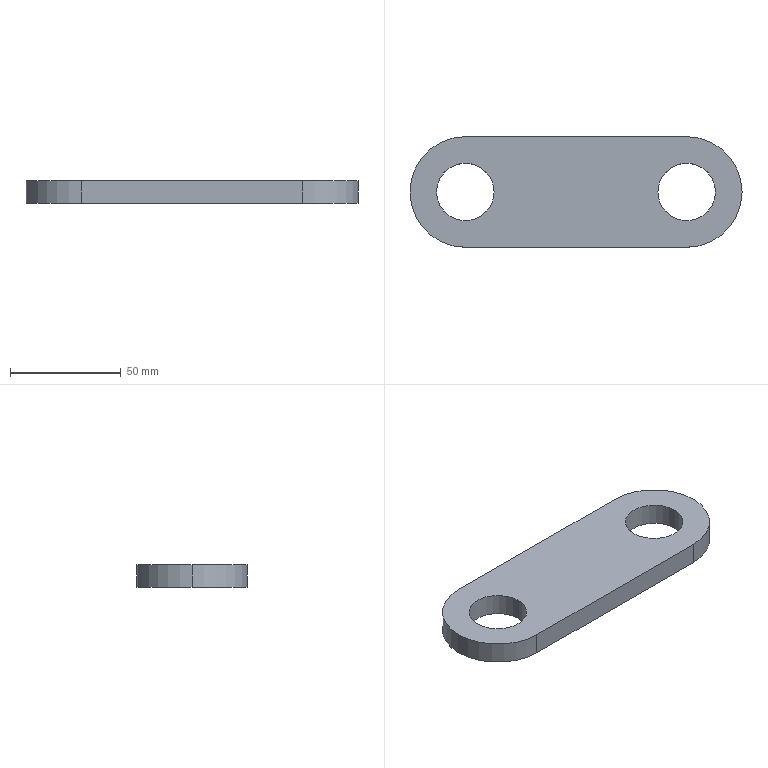Part | STEP file | MYT-A01-P16 | 1 solid | 11 faces | box 150 x 50 x 10 mm | volume 59016 mm3 | cylinder 7 | plane 4 | commonest cylinder face diameters 26 x4 50 x3
STEP:
#1=CARTESIAN_POINT('',(-13.,0.,0.));
#2=VERTEX_POINT('',#1);
#3=CARTESIAN_POINT('',(13.,0.,0.));
#4=VERTEX_POINT('',#3);
#5=CARTESIAN_POINT('',(0.,0.,0.));
#6=DIRECTION('',(0.,0.,1.));
#7=DIRECTION('',(1.,0.,0.));
#8=AXIS2_PLACEMENT_3D('',#5,#6,#7);
#9=CIRCLE('',#8,13.);
#10=EDGE_CURVE('',#2,#4,#9,.T.);
#11=ORIENTED_EDGE('',*,*,#10,.F.);
#12=CARTESIAN_POINT('',(-13.,0.,10.));
#13=VERTEX_POINT('',#12);
#14=CARTESIAN_POINT('',(-13.,0.,0.));
#15=DIRECTION('',(0.,0.,1.));
#16=VECTOR('',#15,1000.);
#17=LINE('',#14,#16);
#18=EDGE_CURVE('',#2,#13,#17,.T.);
#19=ORIENTED_EDGE('',*,*,#18,.T.);
#20=CARTESIAN_POINT('',(13.,0.,10.));
#21=VERTEX_POINT('',#20);
#22=CARTESIAN_POINT('',(0.,0.,10.));
#23=DIRECTION('',(0.,0.,1.));
#24=DIRECTION('',(1.,0.,0.));
#25=AXIS2_PLACEMENT_3D('',#22,#23,#24);
#26=CIRCLE('',#25,13.);
#27=EDGE_CURVE('',#13,#21,#26,.T.);
#28=ORIENTED_EDGE('',*,*,#27,.T.);
#29=CARTESIAN_POINT('',(13.,0.,0.));
#30=DIRECTION('',(0.,0.,1.));
#31=VECTOR('',#30,1000.);
#32=LINE('',#29,#31);
#33=EDGE_CURVE('',#4,#21,#32,.T.);
#34=ORIENTED_EDGE('',*,*,#33,.F.);
#35=EDGE_LOOP('',(#11,#19,#28,#34));
#36=FACE_OUTER_BOUND('',#35,.T.);
#37=CARTESIAN_POINT('',(0.,0.,0.));
#38=DIRECTION('',(0.,0.,1.));
#39=DIRECTION('',(1.,0.,0.));
#40=AXIS2_PLACEMENT_3D('',#37,#38,#39);
#41=CYLINDRICAL_SURFACE('',#40,13.);
#42=ADVANCED_FACE('',(#36),#41,.F.);
#43=CARTESIAN_POINT('',(87.,0.,0.));
#44=VERTEX_POINT('',#43);
#45=CARTESIAN_POINT('',(113.,0.,0.));
#46=VERTEX_POINT('',#45);
#47=CARTESIAN_POINT('',(100.,0.,0.));
#48=DIRECTION('',(0.,0.,1.));
#49=DIRECTION('',(1.,0.,0.));
#50=AXIS2_PLACEMENT_3D('',#47,#48,#49);
#51=CIRCLE('',#50,13.);
#52=EDGE_CURVE('',#44,#46,#51,.T.);
#53=ORIENTED_EDGE('',*,*,#52,.F.);
#54=CARTESIAN_POINT('',(87.,0.,10.));
#55=VERTEX_POINT('',#54);
#56=CARTESIAN_POINT('',(87.,0.,0.));
#57=DIRECTION('',(0.,0.,1.));
#58=VECTOR('',#57,1000.);
#59=LINE('',#56,#58);
#60=EDGE_CURVE('',#44,#55,#59,.T.);
#61=ORIENTED_EDGE('',*,*,#60,.T.);
#62=CARTESIAN_POINT('',(113.,0.,10.));
#63=VERTEX_POINT('',#62);
#64=CARTESIAN_POINT('',(100.,0.,10.));
#65=DIRECTION('',(0.,0.,1.));
#66=DIRECTION('',(1.,0.,0.));
#67=AXIS2_PLACEMENT_3D('',#64,#65,#66);
#68=CIRCLE('',#67,13.);
#69=EDGE_CURVE('',#55,#63,#68,.T.);
#70=ORIENTED_EDGE('',*,*,#69,.T.);
#71=CARTESIAN_POINT('',(113.,0.,0.));
#72=DIRECTION('',(0.,0.,1.));
#73=VECTOR('',#72,1000.);
#74=LINE('',#71,#73);
#75=EDGE_CURVE('',#46,#63,#74,.T.);
#76=ORIENTED_EDGE('',*,*,#75,.F.);
#77=EDGE_LOOP('',(#53,#61,#70,#76));
#78=FACE_OUTER_BOUND('',#77,.T.);
#79=CARTESIAN_POINT('',(100.,0.,0.));
#80=DIRECTION('',(0.,0.,1.));
#81=DIRECTION('',(1.,0.,0.));
#82=AXIS2_PLACEMENT_3D('',#79,#80,#81);
#83=CYLINDRICAL_SURFACE('',#82,13.);
#84=ADVANCED_FACE('',(#78),#83,.F.);
#85=CARTESIAN_POINT('',(-25.,0.,10.));
#86=VERTEX_POINT('',#85);
#87=CARTESIAN_POINT('',(0.,-25.,10.));
#88=VERTEX_POINT('',#87);
#89=CARTESIAN_POINT('',(0.,0.,10.));
#90=DIRECTION('',(0.,0.,1.));
#91=DIRECTION('',(1.,0.,0.));
#92=AXIS2_PLACEMENT_3D('',#89,#90,#91);
#93=CIRCLE('',#92,25.);
#94=EDGE_CURVE('',#86,#88,#93,.T.);
#95=ORIENTED_EDGE('',*,*,#94,.F.);
#96=CARTESIAN_POINT('',(-25.,0.,0.));
#97=VERTEX_POINT('',#96);
#98=CARTESIAN_POINT('',(-25.,0.,10.));
#99=DIRECTION('',(0.,0.,-1.));
#100=VECTOR('',#99,1000.);
#101=LINE('',#98,#100);
#102=EDGE_CURVE('',#86,#97,#101,.T.);
#103=ORIENTED_EDGE('',*,*,#102,.T.);
#104=CARTESIAN_POINT('',(0.,-25.,0.));
#105=VERTEX_POINT('',#104);
#106=CARTESIAN_POINT('',(0.,0.,0.));
#107=DIRECTION('',(0.,0.,1.));
#108=DIRECTION('',(1.,0.,0.));
#109=AXIS2_PLACEMENT_3D('',#106,#107,#108);
#110=CIRCLE('',#109,25.);
#111=EDGE_CURVE('',#97,#105,#110,.T.);
#112=ORIENTED_EDGE('',*,*,#111,.T.);
#113=CARTESIAN_POINT('',(0.,-25.,10.));
#114=DIRECTION('',(0.,0.,-1.));
#115=VECTOR('',#114,1000.);
#116=LINE('',#113,#115);
#117=EDGE_CURVE('',#88,#105,#116,.T.);
#118=ORIENTED_EDGE('',*,*,#117,.F.);
#119=EDGE_LOOP('',(#95,#103,#112,#118));
#120=FACE_OUTER_BOUND('',#119,.T.);
#121=CARTESIAN_POINT('',(0.,0.,10.));
#122=DIRECTION('',(0.,0.,-1.));
#123=DIRECTION('',(-1.,0.,0.));
#124=AXIS2_PLACEMENT_3D('',#121,#122,#123);
#125=CYLINDRICAL_SURFACE('',#124,25.);
#126=ADVANCED_FACE('',(#120),#125,.T.);
#127=ORIENTED_EDGE('',*,*,#102,.F.);
#128=CARTESIAN_POINT('',(0.,25.,10.));
#129=VERTEX_POINT('',#128);
#130=CARTESIAN_POINT('',(0.,0.,10.));
#131=DIRECTION('',(0.,0.,1.));
#132=DIRECTION('',(1.,0.,0.));
#133=AXIS2_PLACEMENT_3D('',#130,#131,#132);
#134=CIRCLE('',#133,25.);
#135=EDGE_CURVE('',#129,#86,#134,.T.);
#136=ORIENTED_EDGE('',*,*,#135,.F.);
#137=CARTESIAN_POINT('',(0.,25.,0.));
#138=VERTEX_POINT('',#137);
#139=CARTESIAN_POINT('',(0.,25.,10.));
#140=DIRECTION('',(0.,0.,-1.));
#141=VECTOR('',#140,1000.);
#142=LINE('',#139,#141);
#143=EDGE_CURVE('',#129,#138,#142,.T.);
#144=ORIENTED_EDGE('',*,*,#143,.T.);
#145=CARTESIAN_POINT('',(0.,0.,0.));
#146=DIRECTION('',(0.,0.,1.));
#147=DIRECTION('',(1.,0.,0.));
#148=AXIS2_PLACEMENT_3D('',#145,#146,#147);
#149=CIRCLE('',#148,25.);
#150=EDGE_CURVE('',#138,#97,#149,.T.);
#151=ORIENTED_EDGE('',*,*,#150,.T.);
#152=EDGE_LOOP('',(#127,#136,#144,#151));
#153=FACE_OUTER_BOUND('',#152,.T.);
#154=CARTESIAN_POINT('',(0.,0.,10.));
#155=DIRECTION('',(0.,0.,-1.));
#156=DIRECTION('',(-1.,0.,0.));
#157=AXIS2_PLACEMENT_3D('',#154,#155,#156);
#158=CYLINDRICAL_SURFACE('',#157,25.);
#159=ADVANCED_FACE('',(#153),#158,.T.);
#160=CARTESIAN_POINT('',(100.,-25.,0.));
#161=VERTEX_POINT('',#160);
#162=CARTESIAN_POINT('',(0.,-25.,0.));
#163=DIRECTION('',(1.,0.,0.));
#164=VECTOR('',#163,1000.);
#165=LINE('',#162,#164);
#166=EDGE_CURVE('',#105,#161,#165,.T.);
#167=ORIENTED_EDGE('',*,*,#166,.T.);
#168=CARTESIAN_POINT('',(100.,-25.,10.));
#169=VERTEX_POINT('',#168);
#170=CARTESIAN_POINT('',(100.,-25.,10.));
#171=DIRECTION('',(0.,0.,-1.));
#172=VECTOR('',#171,1000.);
#173=LINE('',#170,#172);
#174=EDGE_CURVE('',#169,#161,#173,.T.);
#175=ORIENTED_EDGE('',*,*,#174,.F.);
#176=CARTESIAN_POINT('',(0.,-25.,10.));
#177=DIRECTION('',(1.,0.,0.));
#178=VECTOR('',#177,1000.);
#179=LINE('',#176,#178);
#180=EDGE_CURVE('',#88,#169,#179,.T.);
#181=ORIENTED_EDGE('',*,*,#180,.F.);
#182=ORIENTED_EDGE('',*,*,#117,.T.);
#183=EDGE_LOOP('',(#167,#175,#181,#182));
#184=FACE_OUTER_BOUND('',#183,.T.);
#185=CARTESIAN_POINT('',(0.,-25.,10.));
#186=DIRECTION('',(0.,1.,0.));
#187=DIRECTION('',(0.,0.,1.));
#188=AXIS2_PLACEMENT_3D('',#185,#186,#187);
#189=PLANE('',#188);
#190=ADVANCED_FACE('',(#184),#189,.F.);
#191=CARTESIAN_POINT('',(100.,25.,0.));
#192=VERTEX_POINT('',#191);
#193=CARTESIAN_POINT('',(100.,0.,0.));
#194=DIRECTION('',(0.,0.,1.));
#195=DIRECTION('',(1.,0.,0.));
#196=AXIS2_PLACEMENT_3D('',#193,#194,#195);
#197=CIRCLE('',#196,25.);
#198=EDGE_CURVE('',#161,#192,#197,.T.);
#199=ORIENTED_EDGE('',*,*,#198,.T.);
#200=CARTESIAN_POINT('',(100.,25.,10.));
#201=VERTEX_POINT('',#200);
#202=CARTESIAN_POINT('',(100.,25.,10.));
#203=DIRECTION('',(0.,0.,-1.));
#204=VECTOR('',#203,1000.);
#205=LINE('',#202,#204);
#206=EDGE_CURVE('',#201,#192,#205,.T.);
#207=ORIENTED_EDGE('',*,*,#206,.F.);
#208=CARTESIAN_POINT('',(100.,0.,10.));
#209=DIRECTION('',(0.,0.,1.));
#210=DIRECTION('',(1.,0.,0.));
#211=AXIS2_PLACEMENT_3D('',#208,#209,#210);
#212=CIRCLE('',#211,25.);
#213=EDGE_CURVE('',#169,#201,#212,.T.);
#214=ORIENTED_EDGE('',*,*,#213,.F.);
#215=ORIENTED_EDGE('',*,*,#174,.T.);
#216=EDGE_LOOP('',(#199,#207,#214,#215));
#217=FACE_OUTER_BOUND('',#216,.T.);
#218=CARTESIAN_POINT('',(100.,0.,10.));
#219=DIRECTION('',(0.,0.,-1.));
#220=DIRECTION('',(-1.,0.,0.));
#221=AXIS2_PLACEMENT_3D('',#218,#219,#220);
#222=CYLINDRICAL_SURFACE('',#221,25.);
#223=ADVANCED_FACE('',(#217),#222,.T.);
#224=CARTESIAN_POINT('',(0.,25.,0.));
#225=DIRECTION('',(-1.,0.,0.));
#226=VECTOR('',#225,1000.);
#227=LINE('',#224,#226);
#228=EDGE_CURVE('',#192,#138,#227,.T.);
#229=ORIENTED_EDGE('',*,*,#228,.T.);
#230=ORIENTED_EDGE('',*,*,#143,.F.);
#231=CARTESIAN_POINT('',(0.,25.,10.));
#232=DIRECTION('',(-1.,0.,0.));
#233=VECTOR('',#232,1000.);
#234=LINE('',#231,#233);
#235=EDGE_CURVE('',#201,#129,#234,.T.);
#236=ORIENTED_EDGE('',*,*,#235,.F.);
#237=ORIENTED_EDGE('',*,*,#206,.T.);
#238=EDGE_LOOP('',(#229,#230,#236,#237));
#239=FACE_OUTER_BOUND('',#238,.T.);
#240=CARTESIAN_POINT('',(0.,25.,10.));
#241=DIRECTION('',(0.,-1.,0.));
#242=DIRECTION('',(0.,0.,-1.));
#243=AXIS2_PLACEMENT_3D('',#240,#241,#242);
#244=PLANE('',#243);
#245=ADVANCED_FACE('',(#239),#244,.F.);
#246=CARTESIAN_POINT('',(0.,0.,10.));
#247=DIRECTION('',(0.,0.,1.));
#248=DIRECTION('',(1.,0.,0.));
#249=AXIS2_PLACEMENT_3D('',#246,#247,#248);
#250=CIRCLE('',#249,13.);
#251=EDGE_CURVE('',#21,#13,#250,.T.);
#252=ORIENTED_EDGE('',*,*,#251,.F.);
#253=ORIENTED_EDGE('',*,*,#27,.F.);
#254=EDGE_LOOP('',(#252,#253));
#255=FACE_BOUND('',#254,.T.);
#256=CARTESIAN_POINT('',(100.,0.,10.));
#257=DIRECTION('',(0.,0.,1.));
#258=DIRECTION('',(1.,0.,0.));
#259=AXIS2_PLACEMENT_3D('',#256,#257,#258);
#260=CIRCLE('',#259,13.);
#261=EDGE_CURVE('',#63,#55,#260,.T.);
#262=ORIENTED_EDGE('',*,*,#261,.F.);
#263=ORIENTED_EDGE('',*,*,#69,.F.);
#264=EDGE_LOOP('',(#262,#263));
#265=FACE_BOUND('',#264,.T.);
#266=ORIENTED_EDGE('',*,*,#135,.T.);
#267=ORIENTED_EDGE('',*,*,#94,.T.);
#268=ORIENTED_EDGE('',*,*,#180,.T.);
#269=ORIENTED_EDGE('',*,*,#213,.T.);
#270=ORIENTED_EDGE('',*,*,#235,.T.);
#271=EDGE_LOOP('',(#266,#267,#268,#269,#270));
#272=FACE_OUTER_BOUND('',#271,.T.);
#273=CARTESIAN_POINT('',(0.,0.,10.));
#274=DIRECTION('',(0.,0.,1.));
#275=DIRECTION('',(1.,0.,0.));
#276=AXIS2_PLACEMENT_3D('',#273,#274,#275);
#277=PLANE('',#276);
#278=ADVANCED_FACE('',(#255,#265,#272),#277,.T.);
#279=CARTESIAN_POINT('',(0.,0.,0.));
#280=DIRECTION('',(0.,0.,1.));
#281=DIRECTION('',(1.,0.,0.));
#282=AXIS2_PLACEMENT_3D('',#279,#280,#281);
#283=CIRCLE('',#282,13.);
#284=EDGE_CURVE('',#4,#2,#283,.T.);
#285=ORIENTED_EDGE('',*,*,#284,.T.);
#286=ORIENTED_EDGE('',*,*,#10,.T.);
#287=EDGE_LOOP('',(#285,#286));
#288=FACE_BOUND('',#287,.T.);
#289=CARTESIAN_POINT('',(100.,0.,0.));
#290=DIRECTION('',(0.,0.,1.));
#291=DIRECTION('',(1.,0.,0.));
#292=AXIS2_PLACEMENT_3D('',#289,#290,#291);
#293=CIRCLE('',#292,13.);
#294=EDGE_CURVE('',#46,#44,#293,.T.);
#295=ORIENTED_EDGE('',*,*,#294,.T.);
#296=ORIENTED_EDGE('',*,*,#52,.T.);
#297=EDGE_LOOP('',(#295,#296));
#298=FACE_BOUND('',#297,.T.);
#299=ORIENTED_EDGE('',*,*,#150,.F.);
#300=ORIENTED_EDGE('',*,*,#228,.F.);
#301=ORIENTED_EDGE('',*,*,#198,.F.);
#302=ORIENTED_EDGE('',*,*,#166,.F.);
#303=ORIENTED_EDGE('',*,*,#111,.F.);
#304=EDGE_LOOP('',(#299,#300,#301,#302,#303));
#305=FACE_OUTER_BOUND('',#304,.T.);
#306=CARTESIAN_POINT('',(0.,0.,0.));
#307=DIRECTION('',(0.,0.,1.));
#308=DIRECTION('',(1.,0.,0.));
#309=AXIS2_PLACEMENT_3D('',#306,#307,#308);
#310=PLANE('',#309);
#311=ADVANCED_FACE('',(#288,#298,#305),#310,.F.);
#312=ORIENTED_EDGE('',*,*,#60,.F.);
#313=ORIENTED_EDGE('',*,*,#294,.F.);
#314=ORIENTED_EDGE('',*,*,#75,.T.);
#315=ORIENTED_EDGE('',*,*,#261,.T.);
#316=EDGE_LOOP('',(#312,#313,#314,#315));
#317=FACE_OUTER_BOUND('',#316,.T.);
#318=CARTESIAN_POINT('',(100.,0.,0.));
#319=DIRECTION('',(0.,0.,1.));
#320=DIRECTION('',(1.,0.,0.));
#321=AXIS2_PLACEMENT_3D('',#318,#319,#320);
#322=CYLINDRICAL_SURFACE('',#321,13.);
#323=ADVANCED_FACE('',(#317),#322,.F.);
#324=ORIENTED_EDGE('',*,*,#18,.F.);
#325=ORIENTED_EDGE('',*,*,#284,.F.);
#326=ORIENTED_EDGE('',*,*,#33,.T.);
#327=ORIENTED_EDGE('',*,*,#251,.T.);
#328=EDGE_LOOP('',(#324,#325,#326,#327));
#329=FACE_OUTER_BOUND('',#328,.T.);
#330=CARTESIAN_POINT('',(0.,0.,0.));
#331=DIRECTION('',(0.,0.,1.));
#332=DIRECTION('',(1.,0.,0.));
#333=AXIS2_PLACEMENT_3D('',#330,#331,#332);
#334=CYLINDRICAL_SURFACE('',#333,13.);
#335=ADVANCED_FACE('',(#329),#334,.F.);
#336=CLOSED_SHELL('',(#42,#84,#126,#159,#190,#223,#245,#278,#311,#323,#335));
#337=MANIFOLD_SOLID_BREP('',#336);
#338=CARTESIAN_POINT('',(0.,0.,0.));
#339=DIRECTION('',(0.,0.,1.));
#340=DIRECTION('',(1.,0.,0.));
#341=AXIS2_PLACEMENT_3D('',#338,#339,#340);
#342=(LENGTH_UNIT()NAMED_UNIT(*)SI_UNIT(.MILLI.,.METRE.));
#343=UNCERTAINTY_MEASURE_WITH_UNIT(LENGTH_MEASURE(0.00001),#342,'','');
#344=(NAMED_UNIT(*)PLANE_ANGLE_UNIT()SI_UNIT($,.RADIAN.));
#345=(NAMED_UNIT(*)SI_UNIT($,.STERADIAN.)SOLID_ANGLE_UNIT());
#346=(GEOMETRIC_REPRESENTATION_CONTEXT(3)GLOBAL_UNCERTAINTY_ASSIGNED_CONTEXT((#343))GLOBAL_UNIT_ASSIGNED_CONTEXT((#342,#344,#345))REPRESENTATION_CONTEXT('',''));
#347=ADVANCED_BREP_SHAPE_REPRESENTATION('',(#337,#341),#346);